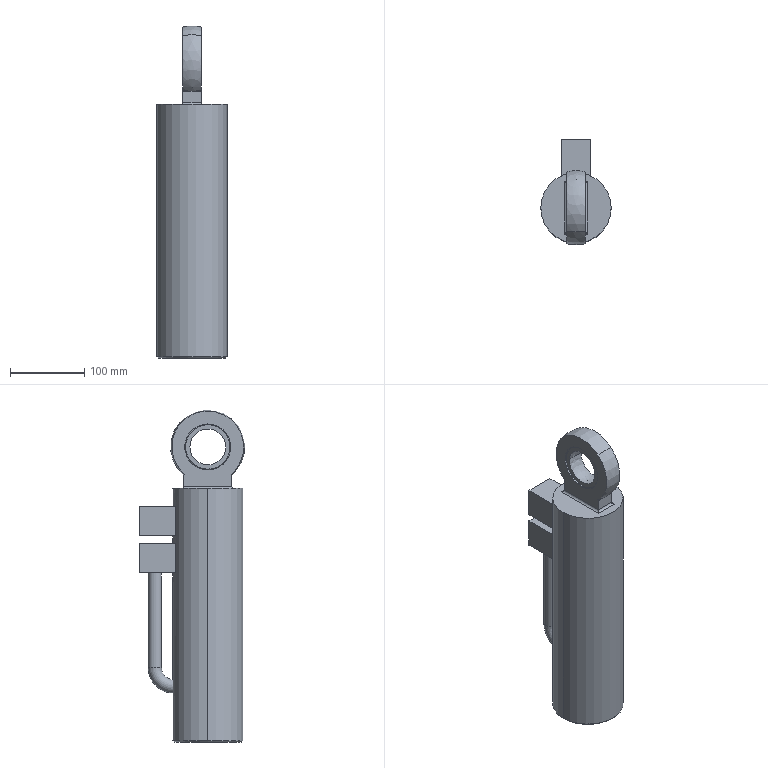Part | SolidWorks | features AEMSimFeature 1 | 1 solid | 64 faces | box 95 x 142.5 x 448 mm | volume 1129896 mm3 | cylinder 26 | plane 24 | torus 8 | sphere 4 | cone 2 | commonest cylinder face diameters 6 x4 13 x4 20.5 x4 62 x4 18 x2 45 x2